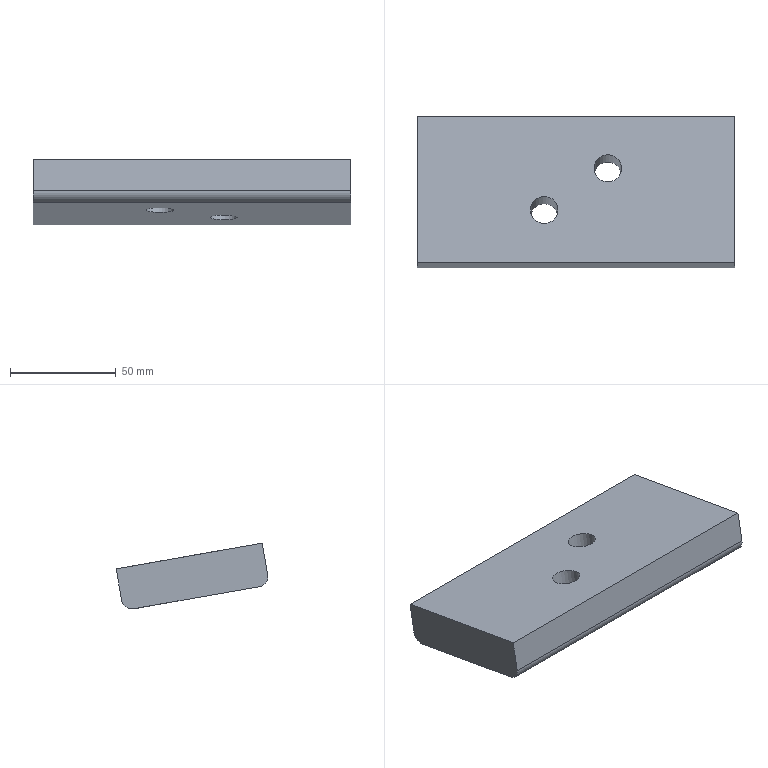Part | NX | features solid 2 | 1 solid | 10 faces | box 150 x 71.617 x 31.059 mm | volume 203081 mm3 | plane 6 | cylinder 4 | commonest cylinder face diameters 10 x2 13 x2
STEP:
#1=CARTESIAN_POINT('',(-22.,-800.561,144.754));
#2=VERTEX_POINT('',#1);
#3=CARTESIAN_POINT('',(-28.5,-800.561,144.754));
#4=DIRECTION('',(0.,0.1736,0.9848));
#5=DIRECTION('',(1.,0.,0.));
#6=AXIS2_PLACEMENT_3D('',#3,#4,#5);
#7=CIRCLE('',#6,6.5);
#8=EDGE_CURVE('',#2,#2,#7,.T.);
#9=ORIENTED_EDGE('',*,*,#8,.T.);
#10=EDGE_LOOP('',(#9));
#11=FACE_BOUND('',#10,.T.);
#12=CARTESIAN_POINT('',(-52.,-820.257,148.227));
#13=VERTEX_POINT('',#12);
#14=CARTESIAN_POINT('',(-58.5,-820.257,148.227));
#15=DIRECTION('',(0.,0.1736,0.9848));
#16=DIRECTION('',(1.,0.,0.));
#17=AXIS2_PLACEMENT_3D('',#14,#15,#16);
#18=CIRCLE('',#17,6.5);
#19=EDGE_CURVE('',#13,#13,#18,.T.);
#20=ORIENTED_EDGE('',*,*,#19,.T.);
#21=EDGE_LOOP('',(#20));
#22=FACE_BOUND('',#21,.T.);
#23=CARTESIAN_POINT('',(-118.5,-780.865,141.281));
#24=VERTEX_POINT('',#23);
#25=CARTESIAN_POINT('',(-118.5,-839.953,151.699));
#26=VERTEX_POINT('',#25);
#27=CARTESIAN_POINT('',(-118.5,-810.409,146.49));
#28=DIRECTION('',(0.,-0.9848,0.1736));
#29=VECTOR('',#28,1000.);
#30=LINE('',#27,#29);
#31=EDGE_CURVE('',#24,#26,#30,.T.);
#32=ORIENTED_EDGE('',*,*,#31,.F.);
#33=CARTESIAN_POINT('',(31.5,-780.865,141.281));
#34=VERTEX_POINT('',#33);
#35=CARTESIAN_POINT('',(-43.5,-780.865,141.281));
#36=DIRECTION('',(-1.,0.,0.));
#37=VECTOR('',#36,1000.);
#38=LINE('',#35,#37);
#39=EDGE_CURVE('',#24,#34,#38,.F.);
#40=ORIENTED_EDGE('',*,*,#39,.T.);
#41=CARTESIAN_POINT('',(31.5,-839.953,151.699));
#42=VERTEX_POINT('',#41);
#43=CARTESIAN_POINT('',(31.5,-810.409,146.49));
#44=DIRECTION('',(0.,0.9848,-0.1736));
#45=VECTOR('',#44,1000.);
#46=LINE('',#43,#45);
#47=EDGE_CURVE('',#42,#34,#46,.T.);
#48=ORIENTED_EDGE('',*,*,#47,.F.);
#49=CARTESIAN_POINT('',(-43.5,-839.953,151.699));
#50=DIRECTION('',(1.,0.,0.));
#51=VECTOR('',#50,1000.);
#52=LINE('',#49,#51);
#53=EDGE_CURVE('',#42,#26,#52,.F.);
#54=ORIENTED_EDGE('',*,*,#53,.T.);
#55=EDGE_LOOP('',(#32,#40,#48,#54));
#56=FACE_BOUND('',#55,.T.);
#57=CARTESIAN_POINT('',(-43.5,-810.409,146.49));
#58=DIRECTION('',(0.,-0.1736,-0.9848));
#59=DIRECTION('',(-1.,0.,0.));
#60=AXIS2_PLACEMENT_3D('',#57,#58,#59);
#61=PLANE('',#60);
#62=ADVANCED_FACE('',(#11,#22,#56),#61,.T.);
#63=CARTESIAN_POINT('',(-118.5,-841.405,172.264));
#64=VERTEX_POINT('',#63);
#65=CARTESIAN_POINT('',(-118.5,-844.009,157.492));
#66=VERTEX_POINT('',#65);
#67=CARTESIAN_POINT('',(-118.5,-841.405,172.264));
#68=DIRECTION('',(0.,-0.1736,-0.9848));
#69=VECTOR('',#68,1000.);
#70=LINE('',#67,#69);
#71=EDGE_CURVE('',#64,#66,#70,.T.);
#72=ORIENTED_EDGE('',*,*,#71,.T.);
#73=CARTESIAN_POINT('',(31.5,-844.009,157.492));
#74=VERTEX_POINT('',#73);
#75=CARTESIAN_POINT('',(-43.5,-844.009,157.492));
#76=DIRECTION('',(1.,0.,0.));
#77=VECTOR('',#76,1000.);
#78=LINE('',#75,#77);
#79=EDGE_CURVE('',#66,#74,#78,.T.);
#80=ORIENTED_EDGE('',*,*,#79,.T.);
#81=CARTESIAN_POINT('',(31.5,-841.405,172.264));
#82=VERTEX_POINT('',#81);
#83=CARTESIAN_POINT('',(31.5,-841.405,172.264));
#84=DIRECTION('',(0.,-0.1736,-0.9848));
#85=VECTOR('',#84,1000.);
#86=LINE('',#83,#85);
#87=EDGE_CURVE('',#82,#74,#86,.T.);
#88=ORIENTED_EDGE('',*,*,#87,.F.);
#89=CARTESIAN_POINT('',(-43.5,-841.405,172.264));
#90=DIRECTION('',(-1.,0.,0.));
#91=VECTOR('',#90,1000.);
#92=LINE('',#89,#91);
#93=EDGE_CURVE('',#82,#64,#92,.T.);
#94=ORIENTED_EDGE('',*,*,#93,.T.);
#95=EDGE_LOOP('',(#72,#80,#88,#94));
#96=FACE_BOUND('',#95,.T.);
#97=CARTESIAN_POINT('',(-43.5,-841.405,172.264));
#98=DIRECTION('',(0.,-0.9848,0.1736));
#99=DIRECTION('',(0.,0.1736,0.9848));
#100=AXIS2_PLACEMENT_3D('',#97,#98,#99);
#101=PLANE('',#100);
#102=ADVANCED_FACE('',(#96),#101,.T.);
#103=ORIENTED_EDGE('',*,*,#47,.T.);
#104=CARTESIAN_POINT('',(31.5,-775.073,145.336));
#105=VERTEX_POINT('',#104);
#106=CARTESIAN_POINT('',(31.5,-779.997,146.205));
#107=DIRECTION('',(1.,0.,0.));
#108=DIRECTION('',(0.,-0.1736,-0.9848));
#109=AXIS2_PLACEMENT_3D('',#106,#107,#108);
#110=CIRCLE('',#109,5.);
#111=EDGE_CURVE('',#34,#105,#110,.T.);
#112=ORIENTED_EDGE('',*,*,#111,.T.);
#113=CARTESIAN_POINT('',(31.5,-772.468,160.109));
#114=VERTEX_POINT('',#113);
#115=CARTESIAN_POINT('',(31.5,-772.468,160.109));
#116=DIRECTION('',(0.,-0.1736,-0.9848));
#117=VECTOR('',#116,1000.);
#118=LINE('',#115,#117);
#119=EDGE_CURVE('',#114,#105,#118,.T.);
#120=ORIENTED_EDGE('',*,*,#119,.F.);
#121=CARTESIAN_POINT('',(31.5,-806.936,166.186));
#122=DIRECTION('',(0.,-0.9848,0.1736));
#123=VECTOR('',#122,1000.);
#124=LINE('',#121,#123);
#125=EDGE_CURVE('',#114,#82,#124,.T.);
#126=ORIENTED_EDGE('',*,*,#125,.T.);
#127=ORIENTED_EDGE('',*,*,#87,.T.);
#128=CARTESIAN_POINT('',(31.5,-839.085,156.624));
#129=DIRECTION('',(1.,0.,0.));
#130=DIRECTION('',(0.,-0.1736,-0.9848));
#131=AXIS2_PLACEMENT_3D('',#128,#129,#130);
#132=CIRCLE('',#131,5.);
#133=EDGE_CURVE('',#74,#42,#132,.T.);
#134=ORIENTED_EDGE('',*,*,#133,.T.);
#135=EDGE_LOOP('',(#103,#112,#120,#126,#127,#134));
#136=FACE_BOUND('',#135,.T.);
#137=CARTESIAN_POINT('',(31.5,-806.936,166.186));
#138=DIRECTION('',(1.,0.,0.));
#139=DIRECTION('',(0.,-0.1736,-0.9848));
#140=AXIS2_PLACEMENT_3D('',#137,#138,#139);
#141=PLANE('',#140);
#142=ADVANCED_FACE('',(#136),#141,.T.);
#143=ORIENTED_EDGE('',*,*,#119,.T.);
#144=CARTESIAN_POINT('',(-118.5,-775.073,145.336));
#145=VERTEX_POINT('',#144);
#146=CARTESIAN_POINT('',(-43.5,-775.073,145.336));
#147=DIRECTION('',(-1.,0.,0.));
#148=VECTOR('',#147,1000.);
#149=LINE('',#146,#148);
#150=EDGE_CURVE('',#105,#145,#149,.T.);
#151=ORIENTED_EDGE('',*,*,#150,.T.);
#152=CARTESIAN_POINT('',(-118.5,-772.468,160.109));
#153=VERTEX_POINT('',#152);
#154=CARTESIAN_POINT('',(-118.5,-772.468,160.109));
#155=DIRECTION('',(0.,-0.1736,-0.9848));
#156=VECTOR('',#155,1000.);
#157=LINE('',#154,#156);
#158=EDGE_CURVE('',#153,#145,#157,.T.);
#159=ORIENTED_EDGE('',*,*,#158,.F.);
#160=CARTESIAN_POINT('',(-43.5,-772.468,160.109));
#161=DIRECTION('',(1.,0.,0.));
#162=VECTOR('',#161,1000.);
#163=LINE('',#160,#162);
#164=EDGE_CURVE('',#153,#114,#163,.T.);
#165=ORIENTED_EDGE('',*,*,#164,.T.);
#166=EDGE_LOOP('',(#143,#151,#159,#165));
#167=FACE_BOUND('',#166,.T.);
#168=CARTESIAN_POINT('',(-43.5,-772.468,160.109));
#169=DIRECTION('',(0.,0.9848,-0.1736));
#170=DIRECTION('',(0.,-0.1736,-0.9848));
#171=AXIS2_PLACEMENT_3D('',#168,#169,#170);
#172=PLANE('',#171);
#173=ADVANCED_FACE('',(#167),#172,.T.);
#174=CARTESIAN_POINT('',(-22.,-797.088,164.45));
#175=VERTEX_POINT('',#174);
#176=CARTESIAN_POINT('',(-28.5,-797.088,164.45));
#177=DIRECTION('',(0.,0.1736,0.9848));
#178=DIRECTION('',(1.,0.,0.));
#179=AXIS2_PLACEMENT_3D('',#176,#177,#178);
#180=CIRCLE('',#179,6.5);
#181=EDGE_CURVE('',#175,#175,#180,.T.);
#182=ORIENTED_EDGE('',*,*,#181,.F.);
#183=EDGE_LOOP('',(#182));
#184=FACE_BOUND('',#183,.T.);
#185=CARTESIAN_POINT('',(-52.,-816.784,167.923));
#186=VERTEX_POINT('',#185);
#187=CARTESIAN_POINT('',(-58.5,-816.784,167.923));
#188=DIRECTION('',(0.,0.1736,0.9848));
#189=DIRECTION('',(1.,0.,0.));
#190=AXIS2_PLACEMENT_3D('',#187,#188,#189);
#191=CIRCLE('',#190,6.5);
#192=EDGE_CURVE('',#186,#186,#191,.T.);
#193=ORIENTED_EDGE('',*,*,#192,.F.);
#194=EDGE_LOOP('',(#193));
#195=FACE_BOUND('',#194,.T.);
#196=CARTESIAN_POINT('',(-118.5,-806.936,166.186));
#197=DIRECTION('',(0.,0.9848,-0.1736));
#198=VECTOR('',#197,1000.);
#199=LINE('',#196,#198);
#200=EDGE_CURVE('',#64,#153,#199,.T.);
#201=ORIENTED_EDGE('',*,*,#200,.F.);
#202=ORIENTED_EDGE('',*,*,#93,.F.);
#203=ORIENTED_EDGE('',*,*,#125,.F.);
#204=ORIENTED_EDGE('',*,*,#164,.F.);
#205=EDGE_LOOP('',(#201,#202,#203,#204));
#206=FACE_BOUND('',#205,.T.);
#207=CARTESIAN_POINT('',(-43.5,-806.936,166.186));
#208=DIRECTION('',(0.,0.1736,0.9848));
#209=DIRECTION('',(1.,0.,0.));
#210=AXIS2_PLACEMENT_3D('',#207,#208,#209);
#211=PLANE('',#210);
#212=ADVANCED_FACE('',(#184,#195,#206),#211,.T.);
#213=ORIENTED_EDGE('',*,*,#158,.T.);
#214=CARTESIAN_POINT('',(-118.5,-779.997,146.205));
#215=DIRECTION('',(-1.,0.,0.));
#216=DIRECTION('',(0.,0.1736,0.9848));
#217=AXIS2_PLACEMENT_3D('',#214,#215,#216);
#218=CIRCLE('',#217,5.);
#219=EDGE_CURVE('',#145,#24,#218,.T.);
#220=ORIENTED_EDGE('',*,*,#219,.T.);
#221=ORIENTED_EDGE('',*,*,#31,.T.);
#222=CARTESIAN_POINT('',(-118.5,-839.085,156.624));
#223=DIRECTION('',(-1.,0.,0.));
#224=DIRECTION('',(0.,0.1736,0.9848));
#225=AXIS2_PLACEMENT_3D('',#222,#223,#224);
#226=CIRCLE('',#225,5.);
#227=EDGE_CURVE('',#26,#66,#226,.T.);
#228=ORIENTED_EDGE('',*,*,#227,.T.);
#229=ORIENTED_EDGE('',*,*,#71,.F.);
#230=ORIENTED_EDGE('',*,*,#200,.T.);
#231=EDGE_LOOP('',(#213,#220,#221,#228,#229,#230));
#232=FACE_BOUND('',#231,.T.);
#233=CARTESIAN_POINT('',(-118.5,-806.936,166.186));
#234=DIRECTION('',(-1.,0.,0.));
#235=DIRECTION('',(0.,0.1736,0.9848));
#236=AXIS2_PLACEMENT_3D('',#233,#234,#235);
#237=PLANE('',#236);
#238=ADVANCED_FACE('',(#232),#237,.T.);
#239=ORIENTED_EDGE('',*,*,#192,.T.);
#240=EDGE_LOOP('',(#239));
#241=FACE_BOUND('',#240,.T.);
#242=ORIENTED_EDGE('',*,*,#19,.F.);
#243=EDGE_LOOP('',(#242));
#244=FACE_BOUND('',#243,.T.);
#245=CARTESIAN_POINT('',(-58.5,-820.257,148.227));
#246=DIRECTION('',(0.,0.1736,0.9848));
#247=DIRECTION('',(1.,0.,0.));
#248=AXIS2_PLACEMENT_3D('',#245,#246,#247);
#249=CYLINDRICAL_SURFACE('',#248,6.5);
#250=ADVANCED_FACE('',(#241,#244),#249,.F.);
#251=ORIENTED_EDGE('',*,*,#181,.T.);
#252=EDGE_LOOP('',(#251));
#253=FACE_BOUND('',#252,.T.);
#254=ORIENTED_EDGE('',*,*,#8,.F.);
#255=EDGE_LOOP('',(#254));
#256=FACE_BOUND('',#255,.T.);
#257=CARTESIAN_POINT('',(-28.5,-800.561,144.754));
#258=DIRECTION('',(0.,0.1736,0.9848));
#259=DIRECTION('',(1.,0.,0.));
#260=AXIS2_PLACEMENT_3D('',#257,#258,#259);
#261=CYLINDRICAL_SURFACE('',#260,6.5);
#262=ADVANCED_FACE('',(#253,#256),#261,.F.);
#263=ORIENTED_EDGE('',*,*,#111,.F.);
#264=ORIENTED_EDGE('',*,*,#39,.F.);
#265=ORIENTED_EDGE('',*,*,#219,.F.);
#266=ORIENTED_EDGE('',*,*,#150,.F.);
#267=EDGE_LOOP('',(#263,#264,#265,#266));
#268=FACE_BOUND('',#267,.T.);
#269=CARTESIAN_POINT('',(-43.5,-779.997,146.205));
#270=DIRECTION('',(-1.,0.,0.));
#271=DIRECTION('',(0.,0.1736,0.9848));
#272=AXIS2_PLACEMENT_3D('',#269,#270,#271);
#273=CYLINDRICAL_SURFACE('',#272,5.);
#274=ADVANCED_FACE('',(#268),#273,.T.);
#275=ORIENTED_EDGE('',*,*,#227,.F.);
#276=ORIENTED_EDGE('',*,*,#53,.F.);
#277=ORIENTED_EDGE('',*,*,#133,.F.);
#278=ORIENTED_EDGE('',*,*,#79,.F.);
#279=EDGE_LOOP('',(#275,#276,#277,#278));
#280=FACE_BOUND('',#279,.T.);
#281=CARTESIAN_POINT('',(-43.5,-839.085,156.624));
#282=DIRECTION('',(1.,0.,0.));
#283=DIRECTION('',(0.,-0.1736,-0.9848));
#284=AXIS2_PLACEMENT_3D('',#281,#282,#283);
#285=CYLINDRICAL_SURFACE('',#284,5.);
#286=ADVANCED_FACE('',(#280),#285,.T.);
#287=CLOSED_SHELL('',(#62,#102,#142,#173,#212,#238,#250,#262,#274,#286));
#288=MANIFOLD_SOLID_BREP('',#287);
#289=(LENGTH_UNIT()NAMED_UNIT(*)SI_UNIT(.MILLI.,.METRE.));
#290=UNCERTAINTY_MEASURE_WITH_UNIT(LENGTH_MEASURE(0.00001),#289,'','');
#291=(NAMED_UNIT(*)PLANE_ANGLE_UNIT()SI_UNIT($,.RADIAN.));
#292=(NAMED_UNIT(*)SI_UNIT($,.STERADIAN.)SOLID_ANGLE_UNIT());
#293=(GEOMETRIC_REPRESENTATION_CONTEXT(3)GLOBAL_UNCERTAINTY_ASSIGNED_CONTEXT((#290))GLOBAL_UNIT_ASSIGNED_CONTEXT((#289,#291,#292))REPRESENTATION_CONTEXT('',''));
#294=ADVANCED_BREP_SHAPE_REPRESENTATION('',(#288),#293);